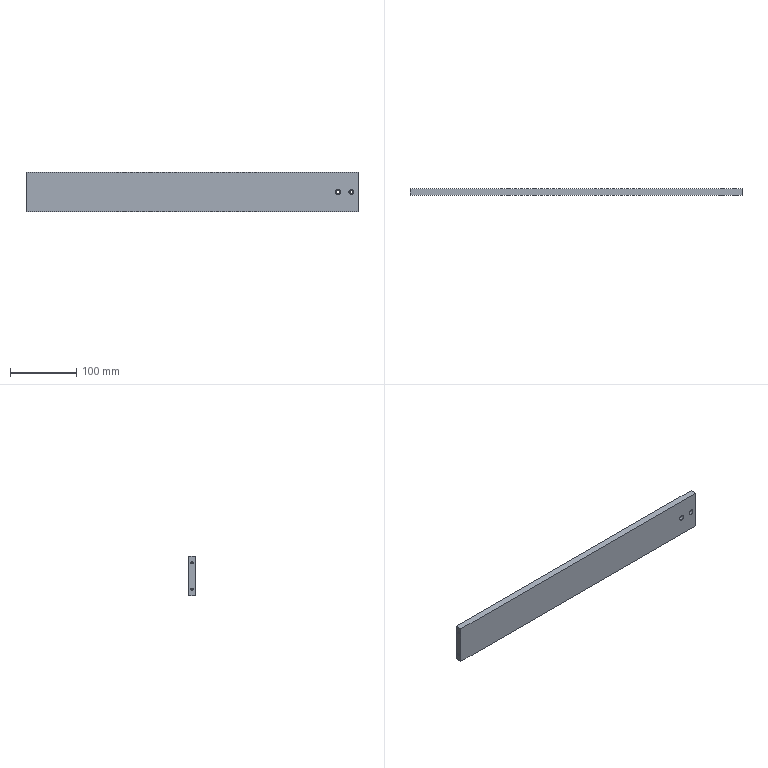Part | STEP file | Camera bracket upright plate | 1 solid | 32 faces | box 500 x 10 x 60 mm | volume 298858 mm3 | cylinder 16 | cone 8 | plane 8 | commonest cylinder face diameters 3.3 x8 4.5 x4 8 x4